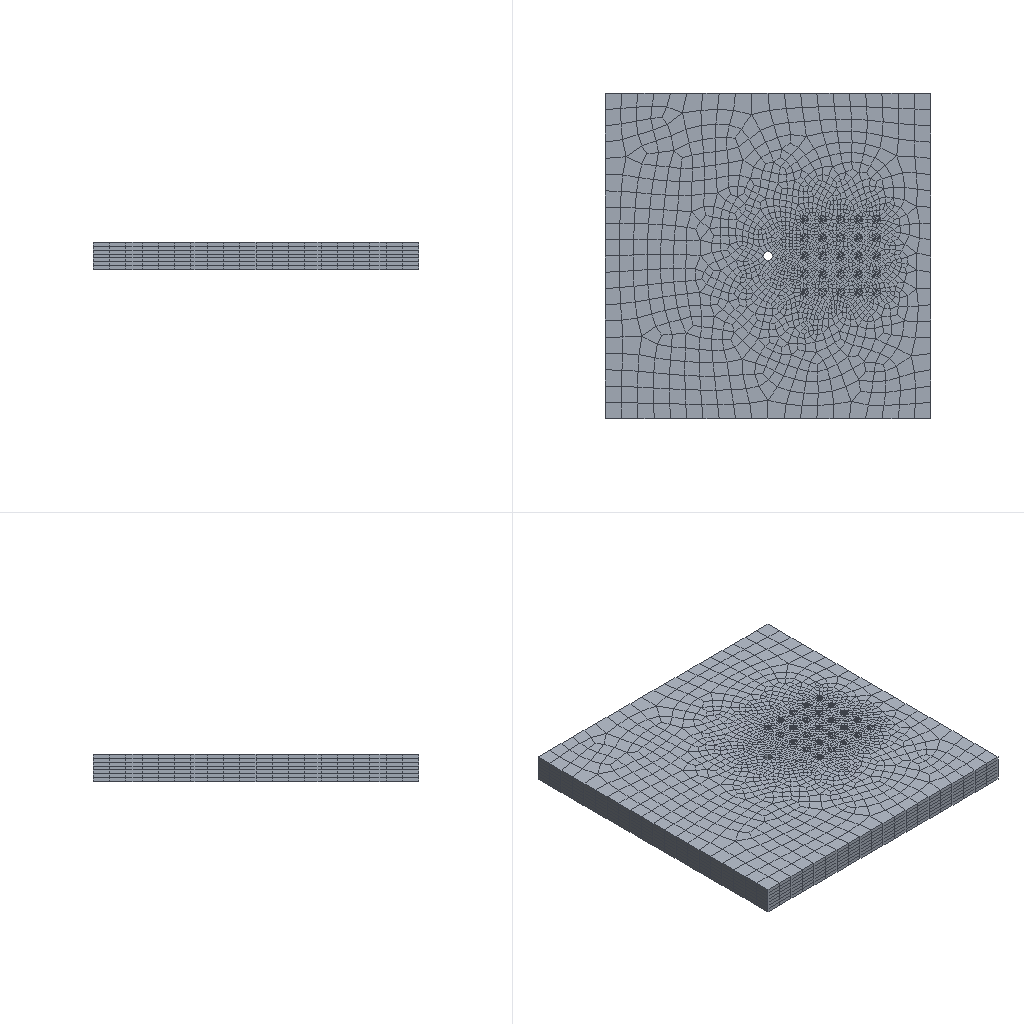Simulation study | abaqus
Set-up summary:
category,name,step,type,value,unit,region
solver,abaqus
solver,version,,,Abaqus/Standard 2020
units,not stated in the deck,,not stated
analysis,deck,,soils,soils
load_step,Step-1,Step-1,soils
load_step,requested,,,1
mesh,nodes,,,33552
mesh,elements,,,26299
element_type,C3D8R,,solid,13860
element_type,C3D8RP,,solid,12439
load,load commands in deck,,count,1
bc,support commands in deck,,count,7
material,SOIL,,in results
material,ZHUANG,,in results
check,setup vs results,,match,"per instance, exact: element labels, types and connectivity; labels of the nodes the elements use; coordinates of those nodes at SINGLE_PRECISION in 1 of 2 instance(s)"
Abaqus input file, long lists of numbers shortened:
*Heading
** Job name: Job-1 Model name: Model-1
** Generated by: Abaqus/CAE 2020
*Preprint, echo=NO, model=NO, history=NO, contact=NO
**
** PARTS
**
*Part, name=Part-1
*Node
      1,   17.1,           0.,           0.
      2,   15.3,           0.,           0.
** (15166 more lines like these left out)
*Element, type=C3D8RP
    1,   289,   327,   307,   328,  2185,  2223,  2203,  2224
    2,   327,   326,   306,   307,  2223,  2222,  2202,  2203
** (12437 more lines like these left out)
*Nset, nset=Set-1, generate
     1,  15168,      1
*Elset, elset=Set-1, generate
     1,  12439,      1
** Section: soil
*Solid Section, elset=Set-1, material=soil
,
*End Part
**
*Part, name=zhuang
*Node
      1,           3.,        -0.25,           0.
      2,           3.,        -0.25,          1.5
** (18382 more lines like these left out)
*Element, type=C3D8R
  1, 7899,  855,  870, 7901,  801,    1,   65,  803
  2, 7910, 7900,  857,  856,  812,  802,   52,   51
** (13858 more lines like these left out)
*Nset, nset=Set-1, generate
     1,  18384,      1
*Elset, elset=Set-1, generate
     1,  13860,      1
** Section: zhuang
*Solid Section, elset=Set-1, material=zhuang
,
*End Part
**
**
** ASSEMBLY
**
*Assembly, name=Assembly
**
*Instance, name=Part-1-1, part=Part-1
*End Instance
**
*Instance, name=zhuang-1, part=zhuang
          9.,          -9.,           0.
*End Instance
**
*Nset, nset=Set-1, instance=Part-1-1
     1,     2,     3,     4,     5,     6,     7,     8,     9,    10,    11,    12,    13,    14,    15,    16
    17,    33,    34,    35,    36,    37,    38,    39,    40,    41,    42,    43,    44,    45,    46,    47
** (19 more lines like these left out)
*Elset, elset=Set-1, instance=Part-1-1
    41,    42,    43,    44,    45,    46,    47,    48,    49,    50,    51,    52,    53,    54,    55,    56
    66,    67,    68,    97,    98,    99,   101,   102,   104,   105,   129,   181,   182,   195,   196,   232
** (16 more lines like these left out)
*Nset, nset=Set-2, instance=Part-1-1
    16,    17,    18,    19,    20,    21,    22,    23,    24,    25,    26,    27,    28,    29,    30,    31
    32,    33,    49,    50,    51,    52,    53,    54,    55,    56,    57,    58,    59,    60,    61,    62
** (19 more lines like these left out)
*Elset, elset=Set-2, instance=Part-1-1
    19,    20,    21,    56,    57,    75,    76,    77,    78,    91,    92,    93,    94,   100,   103,   104
   149,   150,   151,   158,   159,   160,   161,   182,   183,   197,   207,   215,   225,   226,   227,   228
** (16 more lines like these left out)
*Nset, nset=Set-3, instance=Part-1-1, generate
 13273,  15168,      1
*Nset, nset=Set-3, instance=zhuang-1
    2,    4,    6,    8,   10,   12,   14,   16,   18,   20,   22,   24,   26,   28,   30,   32
   34,   36,   38,   40,   42,   44,   46,   48,   50,   66,   67,   68,   69,   70,   71,   72
** (70 more lines like these left out)
*Elset, elset=Set-3, instance=Part-1-1, generate
 10663,  12439,      1
*Elset, elset=Set-3, instance=zhuang-1
   477,   478,   479,   480,   481,   482,   483,   484,   485,   486,   487,   488,   489,   490,   491,   492
   493,   494,   495,   496,   497,   498,   499,   500,   501,   502,   503,   504,   505,   506,   507,   508
** (56 more lines like these left out)
*Nset, nset=Set-4, instance=Part-1-1, generate
    1,  1896,     1
*Elset, elset=Set-4, instance=Part-1-1, generate
    1,  1777,     1
*Nset, nset=Set-5, instance=Part-1-1, generate
     1,  15168,      1
*Nset, nset=Set-5, instance=zhuang-1, generate
     1,  18384,      1
*Elset, elset=Set-5, instance=Part-1-1, generate
     1,  12439,      1
*Elset, elset=Set-5, instance=zhuang-1, generate
     1,  13860,      1
*Nset, nset=Set-6, instance=Part-1-1, generate
     1,  15168,      1
*Elset, elset=Set-6, instance=Part-1-1, generate
     1,  12439,      1
*Nset, nset=Set-7, instance=Part-1-1, generate
 13273,  15168,      1
*Elset, elset=Set-7, instance=Part-1-1, generate
 10663,  12439,      1
*Nset, nset=Set-8, instance=Part-1-1
    65,    66,    67,    68,    69,    70,    71,    72,  1961,  1962,  1963,  1964,  1965,  1966,  1967,  1968
  3857,  3858,  3859,  3860,  3861,  3862,  3863,  3864,  5753,  5754,  5755,  5756,  5757,  5758,  5759,  5760
** (2 more lines like these left out)
*Elset, elset=Set-8, instance=Part-1-1
   114,   116,   119,   234,   236,   798,   833,   834,  1891,  1893,  1896,  2011,  2013,  2575,  2610,  2611
  3668,  3670,  3673,  3788,  3790,  4352,  4387,  4388,  5445,  5447,  5450,  5565,  5567,  6129,  6164,  6165
** (2 more lines like these left out)
*Elset, elset=_m_Surf-1_S4, internal, instance=Part-1-1
    31,    34,    36,    63,    64,    80,    84,   255,   257,   258,   262,   266,   277,   285,   297,   305
   308,   311,   330,   337,   356,   378,   379,   382,   389,   401,   406,   407,   421,   422,   432,   434
** (36 more lines like these left out)
*Elset, elset=_m_Surf-1_S3, internal, instance=Part-1-1
    27,    87,    88,   244,   259,   268,   274,   276,   286,   299,   301,   317,   319,   342,   355,   364
   373,   398,   413,   418,   442,   461,   850,   859,   862,   888,   890,   892,   897,   899,   907,   920
** (15 more lines like these left out)
*Elset, elset=_m_Surf-1_S5, internal, instance=Part-1-1
    29,    33,    65,    86,   248,   275,   298,   306,   310,   316,   324,   328,   329,   345,   369,   387
   414,   420,   427,   642,   649,   700,   802,   805,   806,   813,   816,   841,   844,   860,   868,   878
** (20 more lines like these left out)
*Elset, elset=_m_Surf-1_S6, internal, instance=Part-1-1
    62,    85,   243,   250,   261,   281,   283,   295,   302,   307,   314,   321,   322,   327,   352,   362
   367,   377,   429,   430,   463,   852,   874,   877,   896,   955,  1839,  1862,  2020,  2027,  2038,  2058
** (10 more lines like these left out)
*Surface, type=ELEMENT, name=m_Surf-1
_m_Surf-1_S4, S4
_m_Surf-1_S3, S3
_m_Surf-1_S6, S6
_m_Surf-1_S5, S5
*Elset, elset=_s_Surf-1_S4, internal, instance=zhuang-1
     1,    11,    12,    16,    35,    45,    46,    50,    69,    79,    80,    84,   103,   113,   114,   118
   137,   147,   148,   152,   171,   181,   182,   186,   205,   215,   216,   220,   239,   249,   250,   254
** (107 more lines like these left out)
*Elset, elset=_s_Surf-1_S5, internal, instance=zhuang-1
     2,    28,    36,    62,    70,    96,   104,   130,   138,   164,   172,   198,   206,   232,   240,   266
   274,   300,   308,   334,   342,   368,   376,   402,   410,   436,   444,   470,   478,   504,   512,   533
** (55 more lines like these left out)
*Elset, elset=_s_Surf-1_S3, internal, instance=zhuang-1
     4,    13,    14,    27,    31,    38,    47,    48,    61,    65,    72,    81,    82,    95,    99,   106
   115,   116,   129,   133,   140,   149,   150,   163,   167,   174,   183,   184,   197,   201,   208,   217
** (108 more lines like these left out)
*Elset, elset=_s_Surf-1_S6, internal, instance=zhuang-1
     5,     8,    17,    29,    32,    39,    42,    51,    63,    66,    73,    76,    85,    97,   100,   107
   110,   119,   131,   134,   141,   144,   153,   165,   168,   175,   178,   187,   199,   202,   209,   212
** (99 more lines like these left out)
*Surface, type=ELEMENT, name=s_Surf-1
_s_Surf-1_S4, S4
_s_Surf-1_S5, S5
_s_Surf-1_S6, S6
_s_Surf-1_S3, S3
** Constraint: Constraint-1
*Tie, name=Constraint-1, adjust=yes
s_Surf-1, m_Surf-1
*Nset, nset=Set-7_PP_, internal, instance=Part-1-1, generate
 13273,  15168,      1
*Nset, nset=Set-4_PP_, internal, instance=Part-1-1, generate
    1,  1896,     1
*End Assembly
**
** MATERIALS
**
*Material, name=soil
*Density
1800.,
*Elastic
 1e+08, 0.3
*Gap Flow
 0.001,
*Permeability, specific=9800.
 6e-07, 0.48
*Mohr Coulomb
30., 0.01
*Mohr Coulomb Hardening
13000.,0.
*Material, name=zhuang
*Density
2000.,
*Elastic
 2e+10, 0.15
**
** INTERACTION PROPERTIES
**
*Surface Interaction, name=IntProp-1
1.,
*Friction, slip tolerance=0.005
 0.466,
*Surface Behavior, pressure-overclosure=HARD
**
** PREDEFINED FIELDS
**
** Name: Predefined Field-1   Type: Void ratio
*Initial Conditions, TYPE=RATIO
Set-5, 0.1
** ----------------------------------------------------------------
**
** STEP: Step-1
**
*Step, name=Step-1, nlgeom=YES, inc=100000
*Soils, utol=1.0, cetol=1., stabilize=0.0002, allsdtol=0.05, continue=NO
0.01, 1000., 0.0001, 1000.,
**
** BOUNDARY CONDITIONS
**
** Name: BC-1 Type: 位移/转角
*Boundary
Set-1, 2, 2
** Name: BC-2 Type: 位移/转角
*Boundary
Set-2, 1, 1
** Name: BC-3 Type: 位移/转角
*Boundary
Set-3, 3, 3
** Name: BC-5 Type: 孔隙压力
*Boundary
Set-7_PP_, 8, 8, 1e+06
** Name: BC-6 Type: 位移/转角
*Boundary
Set-8, 1, 1
Set-8, 2, 2
** Name: [REDACTED] : Pore pressure
*Boundary
Set-4_PP_, 8, 8
**
** OUTPUT REQUESTS
**
*Restart, write, frequency=0
**
** FIELD OUTPUT: F-Output-1
**
*Output, field
*Node Output
CF, CFF, POR, RF, RM, RT, RVF, RVT
TF, U, V
*Element Output, directions=YES
ALEAKVRBXFEM, ALEAKVRTXFEM, CRDCUTXFEM, E, FLUVR, FLVEL, GELVR, GFVRXFEM, LE, LEAKVRBXFEM, LEAKVRTXFEM, MISES, MISESMAX, MISESONLY, PE, PEEQ
PEEQMAX, PEEQT, PFOPENXFEM, PFOPENXFEMCOMP, RD, S, SAT, SF, SSAVG, VEEQ, VOIDR, VVF, VVFG, VVFN, YIELDPOT
*Contact Output
CDISP, CSTRESS, PFL, PFLA, PTL, PTLA
**
** HISTORY OUTPUT: H-Output-1
**
*Output, history, variable=PRESELECT
*End Step
Results summary:
result,step,,partial,increments=24 time=23.851/1000.0
result,analysis,,,soils
result,last_loadstep,,,1
result,primary field,,,"U, POR"
result,reaction total,,FX,0.003555,model units
result,reaction total,,FY,0.001308,model units
result,reaction total,,FZ,-0.5509,model units